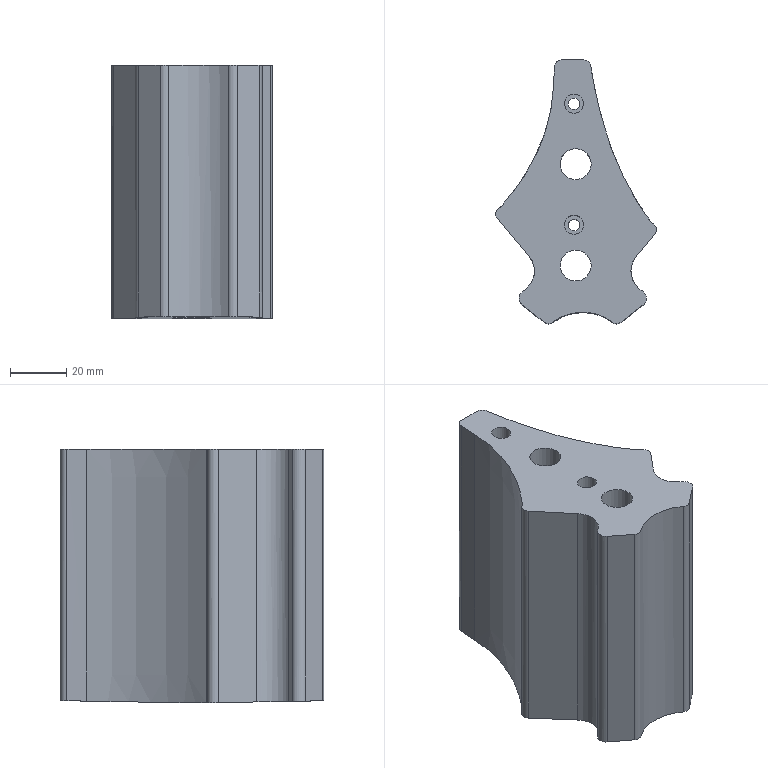Part | STEP file | gslz 2016.10.28-10_id3054_x_t | 1 solid | 39 faces | box 57.01 x 93.6 x 90 mm | volume 227783 mm3 | cylinder 21 | plane 14 | other 3 | spline 1 | commonest cylinder face diameters 5 x8 4.1 x2 6 x2 6.8 x2 11 x2 16 x2